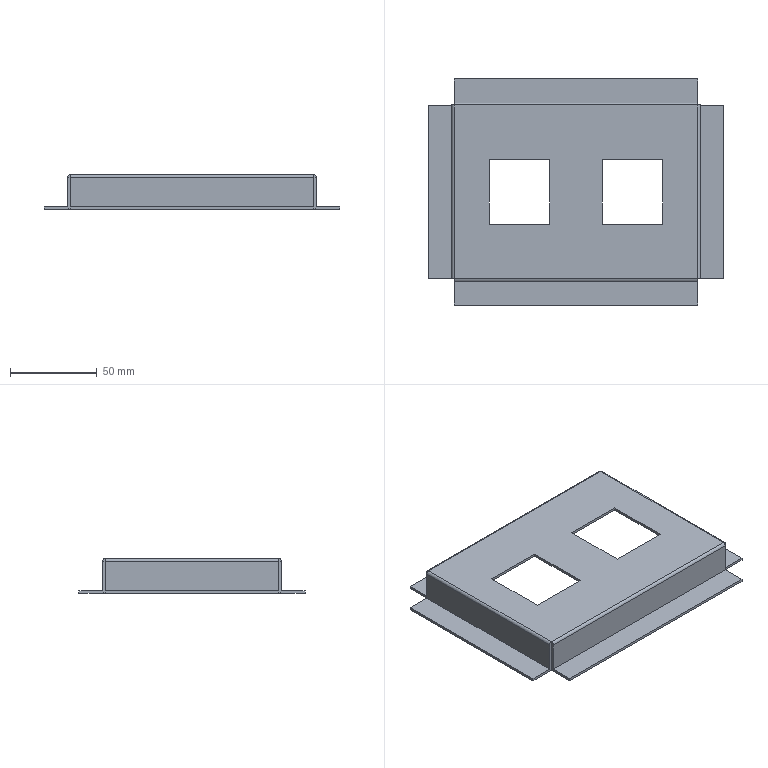Part | NX | features BREP 1 | 1 solid | 58 faces | box 170 x 130 x 20 mm | volume 41003 mm3 | plane 54 | cylinder 4 | commonest cylinder face diameters 3 x4
STEP:
#1=CARTESIAN_POINT('',(-70.,50.,0.));
#2=VERTEX_POINT('',#1);
#3=CARTESIAN_POINT('',(70.,50.,0.));
#4=VERTEX_POINT('',#3);
#5=CARTESIAN_POINT('',(-70.,50.,0.));
#6=DIRECTION('',(1.,0.,0.));
#7=VECTOR('',#6,1000.);
#8=LINE('',#5,#7);
#9=EDGE_CURVE('',#2,#4,#8,.T.);
#10=ORIENTED_EDGE('',*,*,#9,.T.);
#11=CARTESIAN_POINT('',(70.,-50.,0.));
#12=VERTEX_POINT('',#11);
#13=CARTESIAN_POINT('',(70.,50.,0.));
#14=DIRECTION('',(0.,-1.,0.));
#15=VECTOR('',#14,1000.);
#16=LINE('',#13,#15);
#17=EDGE_CURVE('',#4,#12,#16,.T.);
#18=ORIENTED_EDGE('',*,*,#17,.T.);
#19=CARTESIAN_POINT('',(-70.,-50.,0.));
#20=VERTEX_POINT('',#19);
#21=CARTESIAN_POINT('',(70.,-50.,0.));
#22=DIRECTION('',(-1.,0.,0.));
#23=VECTOR('',#22,1000.);
#24=LINE('',#21,#23);
#25=EDGE_CURVE('',#12,#20,#24,.T.);
#26=ORIENTED_EDGE('',*,*,#25,.T.);
#27=CARTESIAN_POINT('',(-70.,-50.,0.));
#28=DIRECTION('',(0.,1.,0.));
#29=VECTOR('',#28,1000.);
#30=LINE('',#27,#29);
#31=EDGE_CURVE('',#20,#2,#30,.T.);
#32=ORIENTED_EDGE('',*,*,#31,.T.);
#33=EDGE_LOOP('',(#10,#18,#26,#32));
#34=FACE_BOUND('',#33,.T.);
#35=CARTESIAN_POINT('',(-15.,18.5,0.));
#36=VERTEX_POINT('',#35);
#37=CARTESIAN_POINT('',(-50.,18.5,0.));
#38=VERTEX_POINT('',#37);
#39=CARTESIAN_POINT('',(-15.,18.5,0.));
#40=DIRECTION('',(-1.,0.,0.));
#41=VECTOR('',#40,1000.);
#42=LINE('',#39,#41);
#43=EDGE_CURVE('',#36,#38,#42,.T.);
#44=ORIENTED_EDGE('',*,*,#43,.T.);
#45=CARTESIAN_POINT('',(-50.,-18.5,0.));
#46=VERTEX_POINT('',#45);
#47=CARTESIAN_POINT('',(-50.,18.5,0.));
#48=DIRECTION('',(0.,-1.,0.));
#49=VECTOR('',#48,1000.);
#50=LINE('',#47,#49);
#51=EDGE_CURVE('',#38,#46,#50,.T.);
#52=ORIENTED_EDGE('',*,*,#51,.T.);
#53=CARTESIAN_POINT('',(-15.,-18.5,0.));
#54=VERTEX_POINT('',#53);
#55=CARTESIAN_POINT('',(-50.,-18.5,0.));
#56=DIRECTION('',(1.,0.,0.));
#57=VECTOR('',#56,1000.);
#58=LINE('',#55,#57);
#59=EDGE_CURVE('',#46,#54,#58,.T.);
#60=ORIENTED_EDGE('',*,*,#59,.T.);
#61=CARTESIAN_POINT('',(-15.,-18.5,0.));
#62=DIRECTION('',(0.,1.,0.));
#63=VECTOR('',#62,1000.);
#64=LINE('',#61,#63);
#65=EDGE_CURVE('',#54,#36,#64,.T.);
#66=ORIENTED_EDGE('',*,*,#65,.T.);
#67=EDGE_LOOP('',(#44,#52,#60,#66));
#68=FACE_BOUND('',#67,.T.);
#69=CARTESIAN_POINT('',(50.,-18.5,0.));
#70=VERTEX_POINT('',#69);
#71=CARTESIAN_POINT('',(15.,-18.5,0.));
#72=VERTEX_POINT('',#71);
#73=CARTESIAN_POINT('',(50.,-18.5,0.));
#74=DIRECTION('',(-1.,0.,0.));
#75=VECTOR('',#74,1000.);
#76=LINE('',#73,#75);
#77=EDGE_CURVE('',#70,#72,#76,.T.);
#78=ORIENTED_EDGE('',*,*,#77,.F.);
#79=CARTESIAN_POINT('',(50.,18.5,0.));
#80=VERTEX_POINT('',#79);
#81=CARTESIAN_POINT('',(50.,18.5,0.));
#82=DIRECTION('',(0.,-1.,0.));
#83=VECTOR('',#82,1000.);
#84=LINE('',#81,#83);
#85=EDGE_CURVE('',#80,#70,#84,.T.);
#86=ORIENTED_EDGE('',*,*,#85,.F.);
#87=CARTESIAN_POINT('',(15.,18.5,0.));
#88=VERTEX_POINT('',#87);
#89=CARTESIAN_POINT('',(15.,18.5,0.));
#90=DIRECTION('',(1.,0.,0.));
#91=VECTOR('',#90,1000.);
#92=LINE('',#89,#91);
#93=EDGE_CURVE('',#88,#80,#92,.T.);
#94=ORIENTED_EDGE('',*,*,#93,.F.);
#95=CARTESIAN_POINT('',(15.,-18.5,0.));
#96=DIRECTION('',(0.,1.,0.));
#97=VECTOR('',#96,1000.);
#98=LINE('',#95,#97);
#99=EDGE_CURVE('',#72,#88,#98,.T.);
#100=ORIENTED_EDGE('',*,*,#99,.F.);
#101=EDGE_LOOP('',(#78,#86,#94,#100));
#102=FACE_BOUND('',#101,.T.);
#103=CARTESIAN_POINT('',(0.,0.,0.));
#104=DIRECTION('',(0.,0.,1.));
#105=DIRECTION('',(1.,0.,0.));
#106=AXIS2_PLACEMENT_3D('',#103,#104,#105);
#107=PLANE('',#106);
#108=ADVANCED_FACE('',(#34,#68,#102),#107,.F.);
#109=CARTESIAN_POINT('',(-70.,-50.,-18.5));
#110=VERTEX_POINT('',#109);
#111=CARTESIAN_POINT('',(-70.,-50.,0.));
#112=DIRECTION('',(0.,0.,-1.));
#113=VECTOR('',#112,1000.);
#114=LINE('',#111,#113);
#115=EDGE_CURVE('',#20,#110,#114,.T.);
#116=ORIENTED_EDGE('',*,*,#115,.T.);
#117=CARTESIAN_POINT('',(-70.,50.,-18.5));
#118=VERTEX_POINT('',#117);
#119=CARTESIAN_POINT('',(-70.,50.,-18.5));
#120=DIRECTION('',(0.,-1.,0.));
#121=VECTOR('',#120,1000.);
#122=LINE('',#119,#121);
#123=EDGE_CURVE('',#118,#110,#122,.T.);
#124=ORIENTED_EDGE('',*,*,#123,.F.);
#125=CARTESIAN_POINT('',(-70.,50.,0.));
#126=DIRECTION('',(0.,0.,-1.));
#127=VECTOR('',#126,1000.);
#128=LINE('',#125,#127);
#129=EDGE_CURVE('',#2,#118,#128,.T.);
#130=ORIENTED_EDGE('',*,*,#129,.F.);
#131=ORIENTED_EDGE('',*,*,#31,.F.);
#132=EDGE_LOOP('',(#116,#124,#130,#131));
#133=FACE_BOUND('',#132,.T.);
#134=CARTESIAN_POINT('',(-70.,-50.,0.));
#135=DIRECTION('',(1.,0.,0.));
#136=DIRECTION('',(0.,1.,0.));
#137=AXIS2_PLACEMENT_3D('',#134,#135,#136);
#138=PLANE('',#137);
#139=ADVANCED_FACE('',(#133),#138,.T.);
#140=CARTESIAN_POINT('',(-71.5,50.,0.));
#141=VERTEX_POINT('',#140);
#142=CARTESIAN_POINT('',(-71.5,50.,0.));
#143=DIRECTION('',(1.,0.,0.));
#144=VECTOR('',#143,1000.);
#145=LINE('',#142,#144);
#146=EDGE_CURVE('',#141,#2,#145,.T.);
#147=ORIENTED_EDGE('',*,*,#146,.T.);
#148=ORIENTED_EDGE('',*,*,#129,.T.);
#149=CARTESIAN_POINT('',(-71.5,50.,-17.));
#150=VERTEX_POINT('',#149);
#151=CARTESIAN_POINT('',(-71.5,50.,-17.));
#152=DIRECTION('',(0.7071,0.,-0.7071));
#153=VECTOR('',#152,1000.);
#154=LINE('',#151,#153);
#155=EDGE_CURVE('',#150,#118,#154,.T.);
#156=ORIENTED_EDGE('',*,*,#155,.F.);
#157=CARTESIAN_POINT('',(-71.5,50.,0.));
#158=DIRECTION('',(0.,0.,-1.));
#159=VECTOR('',#158,1000.);
#160=LINE('',#157,#159);
#161=EDGE_CURVE('',#141,#150,#160,.T.);
#162=ORIENTED_EDGE('',*,*,#161,.F.);
#163=EDGE_LOOP('',(#147,#148,#156,#162));
#164=FACE_BOUND('',#163,.T.);
#165=CARTESIAN_POINT('',(-70.75,50.,-9.25));
#166=DIRECTION('',(0.,1.,0.));
#167=DIRECTION('',(1.,0.,0.));
#168=AXIS2_PLACEMENT_3D('',#165,#166,#167);
#169=PLANE('',#168);
#170=ADVANCED_FACE('',(#164),#169,.T.);
#171=CARTESIAN_POINT('',(-71.5,-50.,0.));
#172=VERTEX_POINT('',#171);
#173=CARTESIAN_POINT('',(-71.5,-50.,0.));
#174=DIRECTION('',(0.,1.,0.));
#175=VECTOR('',#174,1000.);
#176=LINE('',#173,#175);
#177=EDGE_CURVE('',#172,#141,#176,.T.);
#178=ORIENTED_EDGE('',*,*,#177,.T.);
#179=ORIENTED_EDGE('',*,*,#161,.T.);
#180=CARTESIAN_POINT('',(-71.5,-50.,-17.));
#181=VERTEX_POINT('',#180);
#182=CARTESIAN_POINT('',(-71.5,50.,-17.));
#183=DIRECTION('',(0.,-1.,0.));
#184=VECTOR('',#183,1000.);
#185=LINE('',#182,#184);
#186=EDGE_CURVE('',#150,#181,#185,.T.);
#187=ORIENTED_EDGE('',*,*,#186,.T.);
#188=CARTESIAN_POINT('',(-71.5,-50.,0.));
#189=DIRECTION('',(0.,0.,-1.));
#190=VECTOR('',#189,1000.);
#191=LINE('',#188,#190);
#192=EDGE_CURVE('',#172,#181,#191,.T.);
#193=ORIENTED_EDGE('',*,*,#192,.F.);
#194=EDGE_LOOP('',(#178,#179,#187,#193));
#195=FACE_BOUND('',#194,.T.);
#196=CARTESIAN_POINT('',(-71.5,-50.,0.));
#197=DIRECTION('',(1.,0.,0.));
#198=DIRECTION('',(0.,1.,0.));
#199=AXIS2_PLACEMENT_3D('',#196,#197,#198);
#200=PLANE('',#199);
#201=ADVANCED_FACE('',(#195),#200,.F.);
#202=CARTESIAN_POINT('',(-71.5,-50.,-17.));
#203=DIRECTION('',(0.7071,0.,-0.7071));
#204=VECTOR('',#203,1000.);
#205=LINE('',#202,#204);
#206=EDGE_CURVE('',#181,#110,#205,.T.);
#207=ORIENTED_EDGE('',*,*,#206,.T.);
#208=ORIENTED_EDGE('',*,*,#115,.F.);
#209=CARTESIAN_POINT('',(-71.5,-50.,0.));
#210=DIRECTION('',(1.,0.,0.));
#211=VECTOR('',#210,1000.);
#212=LINE('',#209,#211);
#213=EDGE_CURVE('',#172,#20,#212,.T.);
#214=ORIENTED_EDGE('',*,*,#213,.F.);
#215=ORIENTED_EDGE('',*,*,#192,.T.);
#216=EDGE_LOOP('',(#207,#208,#214,#215));
#217=FACE_BOUND('',#216,.T.);
#218=CARTESIAN_POINT('',(-70.75,-50.,-9.25));
#219=DIRECTION('',(0.,1.,0.));
#220=DIRECTION('',(1.,0.,0.));
#221=AXIS2_PLACEMENT_3D('',#218,#219,#220);
#222=PLANE('',#221);
#223=ADVANCED_FACE('',(#217),#222,.F.);
#224=CARTESIAN_POINT('',(-70.,-50.,1.5));
#225=VERTEX_POINT('',#224);
#226=CARTESIAN_POINT('',(-70.,-50.,0.));
#227=DIRECTION('',(0.,0.,1.));
#228=VECTOR('',#227,1000.);
#229=LINE('',#226,#228);
#230=EDGE_CURVE('',#20,#225,#229,.T.);
#231=ORIENTED_EDGE('',*,*,#230,.T.);
#232=CARTESIAN_POINT('',(-70.,-50.,0.));
#233=DIRECTION('',(0.,-1.,0.));
#234=DIRECTION('',(0.,0.,1.));
#235=AXIS2_PLACEMENT_3D('',#232,#233,#234);
#236=CIRCLE('',#235,1.5);
#237=EDGE_CURVE('',#225,#172,#236,.T.);
#238=ORIENTED_EDGE('',*,*,#237,.T.);
#239=ORIENTED_EDGE('',*,*,#213,.T.);
#240=EDGE_LOOP('',(#231,#238,#239));
#241=FACE_BOUND('',#240,.T.);
#242=CARTESIAN_POINT('',(-70.53,-50.,0.5303));
#243=DIRECTION('',(0.,1.,0.));
#244=DIRECTION('',(1.,0.,0.));
#245=AXIS2_PLACEMENT_3D('',#242,#243,#244);
#246=PLANE('',#245);
#247=ADVANCED_FACE('',(#241),#246,.F.);
#248=CARTESIAN_POINT('',(-70.,50.,1.5));
#249=VERTEX_POINT('',#248);
#250=CARTESIAN_POINT('',(-70.,-50.,1.5));
#251=DIRECTION('',(0.,1.,0.));
#252=VECTOR('',#251,1000.);
#253=LINE('',#250,#252);
#254=EDGE_CURVE('',#225,#249,#253,.T.);
#255=ORIENTED_EDGE('',*,*,#254,.T.);
#256=CARTESIAN_POINT('',(-70.,50.,0.));
#257=DIRECTION('',(0.,-1.,0.));
#258=DIRECTION('',(0.,0.,1.));
#259=AXIS2_PLACEMENT_3D('',#256,#257,#258);
#260=CIRCLE('',#259,1.5);
#261=EDGE_CURVE('',#249,#141,#260,.T.);
#262=ORIENTED_EDGE('',*,*,#261,.T.);
#263=ORIENTED_EDGE('',*,*,#177,.F.);
#264=ORIENTED_EDGE('',*,*,#237,.F.);
#265=EDGE_LOOP('',(#255,#262,#263,#264));
#266=FACE_BOUND('',#265,.T.);
#267=CARTESIAN_POINT('',(-70.,-50.,0.));
#268=DIRECTION('',(0.,1.,0.));
#269=DIRECTION('',(-1.,0.,0.));
#270=AXIS2_PLACEMENT_3D('',#267,#268,#269);
#271=CYLINDRICAL_SURFACE('',#270,1.5);
#272=ADVANCED_FACE('',(#266),#271,.T.);
#273=ORIENTED_EDGE('',*,*,#146,.F.);
#274=ORIENTED_EDGE('',*,*,#261,.F.);
#275=CARTESIAN_POINT('',(-70.,50.,0.));
#276=DIRECTION('',(0.,0.,1.));
#277=VECTOR('',#276,1000.);
#278=LINE('',#275,#277);
#279=EDGE_CURVE('',#2,#249,#278,.T.);
#280=ORIENTED_EDGE('',*,*,#279,.F.);
#281=EDGE_LOOP('',(#273,#274,#280));
#282=FACE_BOUND('',#281,.T.);
#283=CARTESIAN_POINT('',(-70.53,50.,0.5303));
#284=DIRECTION('',(0.,1.,0.));
#285=DIRECTION('',(1.,0.,0.));
#286=AXIS2_PLACEMENT_3D('',#283,#284,#285);
#287=PLANE('',#286);
#288=ADVANCED_FACE('',(#282),#287,.T.);
#289=ORIENTED_EDGE('',*,*,#279,.T.);
#290=CARTESIAN_POINT('',(-70.,51.5,0.));
#291=VERTEX_POINT('',#290);
#292=CARTESIAN_POINT('',(-70.,50.,0.));
#293=DIRECTION('',(-1.,0.,0.));
#294=DIRECTION('',(0.,0.,1.));
#295=AXIS2_PLACEMENT_3D('',#292,#293,#294);
#296=CIRCLE('',#295,1.5);
#297=EDGE_CURVE('',#249,#291,#296,.T.);
#298=ORIENTED_EDGE('',*,*,#297,.T.);
#299=CARTESIAN_POINT('',(-70.,51.5,0.));
#300=DIRECTION('',(0.,-1.,0.));
#301=VECTOR('',#300,1000.);
#302=LINE('',#299,#301);
#303=EDGE_CURVE('',#291,#2,#302,.T.);
#304=ORIENTED_EDGE('',*,*,#303,.T.);
#305=EDGE_LOOP('',(#289,#298,#304));
#306=FACE_BOUND('',#305,.T.);
#307=CARTESIAN_POINT('',(-70.,50.53,0.5303));
#308=DIRECTION('',(1.,0.,0.));
#309=DIRECTION('',(0.,1.,0.));
#310=AXIS2_PLACEMENT_3D('',#307,#308,#309);
#311=PLANE('',#310);
#312=ADVANCED_FACE('',(#306),#311,.F.);
#313=CARTESIAN_POINT('',(-70.,51.5,-17.));
#314=VERTEX_POINT('',#313);
#315=CARTESIAN_POINT('',(-70.,50.,-18.5));
#316=VERTEX_POINT('',#315);
#317=CARTESIAN_POINT('',(-70.,51.5,-17.));
#318=DIRECTION('',(0.,-0.7071,-0.7071));
#319=VECTOR('',#318,1000.);
#320=LINE('',#317,#319);
#321=EDGE_CURVE('',#314,#316,#320,.T.);
#322=ORIENTED_EDGE('',*,*,#321,.T.);
#323=CARTESIAN_POINT('',(-70.,50.,0.));
#324=DIRECTION('',(0.,0.,-1.));
#325=VECTOR('',#324,1000.);
#326=LINE('',#323,#325);
#327=EDGE_CURVE('',#2,#316,#326,.T.);
#328=ORIENTED_EDGE('',*,*,#327,.F.);
#329=ORIENTED_EDGE('',*,*,#303,.F.);
#330=CARTESIAN_POINT('',(-70.,51.5,0.));
#331=DIRECTION('',(0.,0.,-1.));
#332=VECTOR('',#331,1000.);
#333=LINE('',#330,#332);
#334=EDGE_CURVE('',#291,#314,#333,.T.);
#335=ORIENTED_EDGE('',*,*,#334,.T.);
#336=EDGE_LOOP('',(#322,#328,#329,#335));
#337=FACE_BOUND('',#336,.T.);
#338=CARTESIAN_POINT('',(-70.,50.75,-9.25));
#339=DIRECTION('',(1.,0.,0.));
#340=DIRECTION('',(0.,1.,0.));
#341=AXIS2_PLACEMENT_3D('',#338,#339,#340);
#342=PLANE('',#341);
#343=ADVANCED_FACE('',(#337),#342,.F.);
#344=CARTESIAN_POINT('',(70.,51.5,0.));
#345=VERTEX_POINT('',#344);
#346=CARTESIAN_POINT('',(-70.,51.5,0.));
#347=DIRECTION('',(1.,0.,0.));
#348=VECTOR('',#347,1000.);
#349=LINE('',#346,#348);
#350=EDGE_CURVE('',#291,#345,#349,.T.);
#351=ORIENTED_EDGE('',*,*,#350,.T.);
#352=CARTESIAN_POINT('',(70.,51.5,-17.));
#353=VERTEX_POINT('',#352);
#354=CARTESIAN_POINT('',(70.,51.5,0.));
#355=DIRECTION('',(0.,0.,-1.));
#356=VECTOR('',#355,1000.);
#357=LINE('',#354,#356);
#358=EDGE_CURVE('',#345,#353,#357,.T.);
#359=ORIENTED_EDGE('',*,*,#358,.T.);
#360=CARTESIAN_POINT('',(70.,51.5,-17.));
#361=DIRECTION('',(-1.,0.,0.));
#362=VECTOR('',#361,1000.);
#363=LINE('',#360,#362);
#364=EDGE_CURVE('',#353,#314,#363,.T.);
#365=ORIENTED_EDGE('',*,*,#364,.T.);
#366=ORIENTED_EDGE('',*,*,#334,.F.);
#367=EDGE_LOOP('',(#351,#359,#365,#366));
#368=FACE_BOUND('',#367,.T.);
#369=CARTESIAN_POINT('',(-70.,51.5,0.));
#370=DIRECTION('',(0.,-1.,0.));
#371=DIRECTION('',(0.,0.,-1.));
#372=AXIS2_PLACEMENT_3D('',#369,#370,#371);
#373=PLANE('',#372);
#374=ADVANCED_FACE('',(#368),#373,.F.);
#375=ORIENTED_EDGE('',*,*,#364,.F.);
#376=CARTESIAN_POINT('',(70.,65.,-17.));
#377=VERTEX_POINT('',#376);
#378=CARTESIAN_POINT('',(70.,65.,-17.));
#379=DIRECTION('',(0.,-1.,0.));
#380=VECTOR('',#379,1000.);
#381=LINE('',#378,#380);
#382=EDGE_CURVE('',#377,#353,#381,.T.);
#383=ORIENTED_EDGE('',*,*,#382,.F.);
#384=CARTESIAN_POINT('',(-70.,65.,-17.));
#385=VERTEX_POINT('',#384);
#386=CARTESIAN_POINT('',(-70.,65.,-17.));
#387=DIRECTION('',(1.,0.,0.));
#388=VECTOR('',#387,1000.);
#389=LINE('',#386,#388);
#390=EDGE_CURVE('',#385,#377,#389,.T.);
#391=ORIENTED_EDGE('',*,*,#390,.F.);
#392=CARTESIAN_POINT('',(-70.,51.5,-17.));
#393=DIRECTION('',(0.,1.,0.));
#394=VECTOR('',#393,1000.);
#395=LINE('',#392,#394);
#396=EDGE_CURVE('',#314,#385,#395,.T.);
#397=ORIENTED_EDGE('',*,*,#396,.F.);
#398=EDGE_LOOP('',(#375,#383,#391,#397));
#399=FACE_BOUND('',#398,.T.);
#400=CARTESIAN_POINT('',(-70.,50.,-17.));
#401=DIRECTION('',(0.,0.,-1.));
#402=DIRECTION('',(0.,-1.,0.));
#403=AXIS2_PLACEMENT_3D('',#400,#401,#402);
#404=PLANE('',#403);
#405=ADVANCED_FACE('',(#399),#404,.F.);
#406=CARTESIAN_POINT('',(-70.,65.,-18.5));
#407=VERTEX_POINT('',#406);
#408=CARTESIAN_POINT('',(-70.,65.,-18.5));
#409=DIRECTION('',(0.,0.,1.));
#410=VECTOR('',#409,1000.);
#411=LINE('',#408,#410);
#412=EDGE_CURVE('',#407,#385,#411,.T.);
#413=ORIENTED_EDGE('',*,*,#412,.F.);
#414=CARTESIAN_POINT('',(-70.,50.,-18.5));
#415=DIRECTION('',(0.,1.,0.));
#416=VECTOR('',#415,1000.);
#417=LINE('',#414,#416);
#418=EDGE_CURVE('',#316,#407,#417,.T.);
#419=ORIENTED_EDGE('',*,*,#418,.F.);
#420=ORIENTED_EDGE('',*,*,#321,.F.);
#421=ORIENTED_EDGE('',*,*,#396,.T.);
#422=EDGE_LOOP('',(#413,#419,#420,#421));
#423=FACE_BOUND('',#422,.T.);
#424=CARTESIAN_POINT('',(-70.,57.5,-17.75));
#425=DIRECTION('',(-1.,0.,0.));
#426=DIRECTION('',(0.,0.,1.));
#427=AXIS2_PLACEMENT_3D('',#424,#425,#426);
#428=PLANE('',#427);
#429=ADVANCED_FACE('',(#423),#428,.T.);
#430=CARTESIAN_POINT('',(70.,65.,-18.5));
#431=VERTEX_POINT('',#430);
#432=CARTESIAN_POINT('',(-70.,65.,-18.5));
#433=DIRECTION('',(1.,0.,0.));
#434=VECTOR('',#433,1000.);
#435=LINE('',#432,#434);
#436=EDGE_CURVE('',#407,#431,#435,.T.);
#437=ORIENTED_EDGE('',*,*,#436,.T.);
#438=CARTESIAN_POINT('',(70.,50.,-18.5));
#439=VERTEX_POINT('',#438);
#440=CARTESIAN_POINT('',(70.,65.,-18.5));
#441=DIRECTION('',(0.,-1.,0.));
#442=VECTOR('',#441,1000.);
#443=LINE('',#440,#442);
#444=EDGE_CURVE('',#431,#439,#443,.T.);
#445=ORIENTED_EDGE('',*,*,#444,.T.);
#446=CARTESIAN_POINT('',(70.,50.,-18.5));
#447=DIRECTION('',(-1.,0.,0.));
#448=VECTOR('',#447,1000.);
#449=LINE('',#446,#448);
#450=EDGE_CURVE('',#439,#316,#449,.T.);
#451=ORIENTED_EDGE('',*,*,#450,.T.);
#452=ORIENTED_EDGE('',*,*,#418,.T.);
#453=EDGE_LOOP('',(#437,#445,#451,#452));
#454=FACE_BOUND('',#453,.T.);
#455=CARTESIAN_POINT('',(-70.,50.,-18.5));
#456=DIRECTION('',(0.,0.,-1.));
#457=DIRECTION('',(0.,-1.,0.));
#458=AXIS2_PLACEMENT_3D('',#455,#456,#457);
#459=PLANE('',#458);
#460=ADVANCED_FACE('',(#454),#459,.T.);
#461=ORIENTED_EDGE('',*,*,#327,.T.);
#462=ORIENTED_EDGE('',*,*,#450,.F.);
#463=CARTESIAN_POINT('',(70.,50.,0.));
#464=DIRECTION('',(0.,0.,-1.));
#465=VECTOR('',#464,1000.);
#466=LINE('',#463,#465);
#467=EDGE_CURVE('',#4,#439,#466,.T.);
#468=ORIENTED_EDGE('',*,*,#467,.F.);
#469=ORIENTED_EDGE('',*,*,#9,.F.);
#470=EDGE_LOOP('',(#461,#462,#468,#469));
#471=FACE_BOUND('',#470,.T.);
#472=CARTESIAN_POINT('',(-70.,50.,0.));
#473=DIRECTION('',(0.,-1.,0.));
#474=DIRECTION('',(0.,0.,-1.));
#475=AXIS2_PLACEMENT_3D('',#472,#473,#474);
#476=PLANE('',#475);
#477=ADVANCED_FACE('',(#471),#476,.T.);
#478=CARTESIAN_POINT('',(70.,51.5,0.));
#479=DIRECTION('',(0.,-1.,0.));
#480=VECTOR('',#479,1000.);
#481=LINE('',#478,#480);
#482=EDGE_CURVE('',#345,#4,#481,.T.);
#483=ORIENTED_EDGE('',*,*,#482,.T.);
#484=ORIENTED_EDGE('',*,*,#467,.T.);
#485=CARTESIAN_POINT('',(70.,51.5,-17.));
#486=DIRECTION('',(0.,-0.7071,-0.7071));
#487=VECTOR('',#486,1000.);
#488=LINE('',#485,#487);
#489=EDGE_CURVE('',#353,#439,#488,.T.);
#490=ORIENTED_EDGE('',*,*,#489,.F.);
#491=ORIENTED_EDGE('',*,*,#358,.F.);
#492=EDGE_LOOP('',(#483,#484,#490,#491));
#493=FACE_BOUND('',#492,.T.);
#494=CARTESIAN_POINT('',(70.,50.75,-9.25));
#495=DIRECTION('',(1.,0.,0.));
#496=DIRECTION('',(0.,1.,0.));
#497=AXIS2_PLACEMENT_3D('',#494,#495,#496);
#498=PLANE('',#497);
#499=ADVANCED_FACE('',(#493),#498,.T.);
#500=ORIENTED_EDGE('',*,*,#489,.T.);
#501=ORIENTED_EDGE('',*,*,#444,.F.);
#502=CARTESIAN_POINT('',(70.,65.,-18.5));
#503=DIRECTION('',(0.,0.,1.));
#504=VECTOR('',#503,1000.);
#505=LINE('',#502,#504);
#506=EDGE_CURVE('',#431,#377,#505,.T.);
#507=ORIENTED_EDGE('',*,*,#506,.T.);
#508=ORIENTED_EDGE('',*,*,#382,.T.);
#509=EDGE_LOOP('',(#500,#501,#507,#508));
#510=FACE_BOUND('',#509,.T.);
#511=CARTESIAN_POINT('',(70.,57.5,-17.75));
#512=DIRECTION('',(1.,0.,0.));
#513=DIRECTION('',(0.,1.,0.));
#514=AXIS2_PLACEMENT_3D('',#511,#512,#513);
#515=PLANE('',#514);
#516=ADVANCED_FACE('',(#510),#515,.T.);
#517=ORIENTED_EDGE('',*,*,#412,.T.);
#518=ORIENTED_EDGE('',*,*,#390,.T.);
#519=ORIENTED_EDGE('',*,*,#506,.F.);
#520=ORIENTED_EDGE('',*,*,#436,.F.);
#521=EDGE_LOOP('',(#517,#518,#519,#520));
#522=FACE_BOUND('',#521,.T.);
#523=CARTESIAN_POINT('',(0.,65.,-17.75));
#524=DIRECTION('',(0.,1.,0.));
#525=DIRECTION('',(1.,0.,0.));
#526=AXIS2_PLACEMENT_3D('',#523,#524,#525);
#527=PLANE('',#526);
#528=ADVANCED_FACE('',(#522),#527,.T.);
#529=ORIENTED_EDGE('',*,*,#482,.F.);
#530=CARTESIAN_POINT('',(70.,50.,1.5));
#531=VERTEX_POINT('',#530);
#532=CARTESIAN_POINT('',(70.,50.,0.));
#533=DIRECTION('',(-1.,0.,0.));
#534=DIRECTION('',(0.,0.,1.));
#535=AXIS2_PLACEMENT_3D('',#532,#533,#534);
#536=CIRCLE('',#535,1.5);
#537=EDGE_CURVE('',#531,#345,#536,.T.);
#538=ORIENTED_EDGE('',*,*,#537,.F.);
#539=CARTESIAN_POINT('',(70.,50.,0.));
#540=DIRECTION('',(0.,0.,1.));
#541=VECTOR('',#540,1000.);
#542=LINE('',#539,#541);
#543=EDGE_CURVE('',#4,#531,#542,.T.);
#544=ORIENTED_EDGE('',*,*,#543,.F.);
#545=EDGE_LOOP('',(#529,#538,#544));
#546=FACE_BOUND('',#545,.T.);
#547=CARTESIAN_POINT('',(70.,50.53,0.5303));
#548=DIRECTION('',(1.,0.,0.));
#549=DIRECTION('',(0.,1.,0.));
#550=AXIS2_PLACEMENT_3D('',#547,#548,#549);
#551=PLANE('',#550);
#552=ADVANCED_FACE('',(#546),#551,.T.);
#553=ORIENTED_EDGE('',*,*,#543,.T.);
#554=CARTESIAN_POINT('',(71.5,50.,0.));
#555=VERTEX_POINT('',#554);
#556=CARTESIAN_POINT('',(70.,50.,0.));
#557=DIRECTION('',(0.,1.,0.));
#558=DIRECTION('',(0.,0.,1.));
#559=AXIS2_PLACEMENT_3D('',#556,#557,#558);
#560=CIRCLE('',#559,1.5);
#561=EDGE_CURVE('',#531,#555,#560,.T.);
#562=ORIENTED_EDGE('',*,*,#561,.T.);
#563=CARTESIAN_POINT('',(71.5,50.,0.));
#564=DIRECTION('',(-1.,0.,0.));
#565=VECTOR('',#564,1000.);
#566=LINE('',#563,#565);
#567=EDGE_CURVE('',#555,#4,#566,.T.);
#568=ORIENTED_EDGE('',*,*,#567,.T.);
#569=EDGE_LOOP('',(#553,#562,#568));
#570=FACE_BOUND('',#569,.T.);
#571=CARTESIAN_POINT('',(70.53,50.,0.5303));
#572=DIRECTION('',(0.,-1.,0.));
#573=DIRECTION('',(0.,0.,-1.));
#574=AXIS2_PLACEMENT_3D('',#571,#572,#573);
#575=PLANE('',#574);
#576=ADVANCED_FACE('',(#570),#575,.F.);
#577=CARTESIAN_POINT('',(71.5,50.,-17.));
#578=VERTEX_POINT('',#577);
#579=CARTESIAN_POINT('',(70.,50.,-18.5));
#580=VERTEX_POINT('',#579);
#581=CARTESIAN_POINT('',(71.5,50.,-17.));
#582=DIRECTION('',(-0.7071,0.,-0.7071));
#583=VECTOR('',#582,1000.);
#584=LINE('',#581,#583);
#585=EDGE_CURVE('',#578,#580,#584,.T.);
#586=ORIENTED_EDGE('',*,*,#585,.T.);
#587=CARTESIAN_POINT('',(70.,50.,0.));
#588=DIRECTION('',(0.,0.,-1.));
#589=VECTOR('',#588,1000.);
#590=LINE('',#587,#589);
#591=EDGE_CURVE('',#4,#580,#590,.T.);
#592=ORIENTED_EDGE('',*,*,#591,.F.);
#593=ORIENTED_EDGE('',*,*,#567,.F.);
#594=CARTESIAN_POINT('',(71.5,50.,0.));
#595=DIRECTION('',(0.,0.,-1.));
#596=VECTOR('',#595,1000.);
#597=LINE('',#594,#596);
#598=EDGE_CURVE('',#555,#578,#597,.T.);
#599=ORIENTED_EDGE('',*,*,#598,.T.);
#600=EDGE_LOOP('',(#586,#592,#593,#599));
#601=FACE_BOUND('',#600,.T.);
#602=CARTESIAN_POINT('',(70.75,50.,-9.25));
#603=DIRECTION('',(0.,-1.,0.));
#604=DIRECTION('',(0.,0.,-1.));
#605=AXIS2_PLACEMENT_3D('',#602,#603,#604);
#606=PLANE('',#605);
#607=ADVANCED_FACE('',(#601),#606,.F.);
#608=CARTESIAN_POINT('',(71.5,-50.,0.));
#609=VERTEX_POINT('',#608);
#610=CARTESIAN_POINT('',(71.5,50.,0.));
#611=DIRECTION('',(0.,-1.,0.));
#612=VECTOR('',#611,1000.);
#613=LINE('',#610,#612);
#614=EDGE_CURVE('',#555,#609,#613,.T.);
#615=ORIENTED_EDGE('',*,*,#614,.T.);
#616=CARTESIAN_POINT('',(71.5,-50.,-17.));
#617=VERTEX_POINT('',#616);
#618=CARTESIAN_POINT('',(71.5,-50.,0.));
#619=DIRECTION('',(0.,0.,-1.));
#620=VECTOR('',#619,1000.);
#621=LINE('',#618,#620);
#622=EDGE_CURVE('',#609,#617,#621,.T.);
#623=ORIENTED_EDGE('',*,*,#622,.T.);
#624=CARTESIAN_POINT('',(71.5,50.,-17.));
#625=DIRECTION('',(0.,-1.,0.));
#626=VECTOR('',#625,1000.);
#627=LINE('',#624,#626);
#628=EDGE_CURVE('',#578,#617,#627,.T.);
#629=ORIENTED_EDGE('',*,*,#628,.F.);
#630=ORIENTED_EDGE('',*,*,#598,.F.);
#631=EDGE_LOOP('',(#615,#623,#629,#630));
#632=FACE_BOUND('',#631,.T.);
#633=CARTESIAN_POINT('',(71.5,50.,0.));
#634=DIRECTION('',(-1.,0.,0.));
#635=DIRECTION('',(0.,0.,1.));
#636=AXIS2_PLACEMENT_3D('',#633,#634,#635);
#637=PLANE('',#636);
#638=ADVANCED_FACE('',(#632),#637,.F.);
#639=CARTESIAN_POINT('',(85.,-50.,-17.));
#640=VERTEX_POINT('',#639);
#641=CARTESIAN_POINT('',(85.,50.,-17.));
#642=VERTEX_POINT('',#641);
#643=CARTESIAN_POINT('',(85.,-50.,-17.));
#644=DIRECTION('',(0.,1.,0.));
#645=VECTOR('',#644,1000.);
#646=LINE('',#643,#645);
#647=EDGE_CURVE('',#640,#642,#646,.T.);
#648=ORIENTED_EDGE('',*,*,#647,.T.);
#649=CARTESIAN_POINT('',(85.,50.,-17.));
#650=DIRECTION('',(-1.,0.,0.));
#651=VECTOR('',#650,1000.);
#652=LINE('',#649,#651);
#653=EDGE_CURVE('',#642,#578,#652,.T.);
#654=ORIENTED_EDGE('',*,*,#653,.T.);
#655=ORIENTED_EDGE('',*,*,#628,.T.);
#656=CARTESIAN_POINT('',(71.5,-50.,-17.));
#657=DIRECTION('',(1.,0.,0.));
#658=VECTOR('',#657,1000.);
#659=LINE('',#656,#658);
#660=EDGE_CURVE('',#617,#640,#659,.T.);
#661=ORIENTED_EDGE('',*,*,#660,.T.);
#662=EDGE_LOOP('',(#648,#654,#655,#661));
#663=FACE_BOUND('',#662,.T.);
#664=CARTESIAN_POINT('',(70.,-50.,-17.));
#665=DIRECTION('',(0.,0.,1.));
#666=DIRECTION('',(1.,0.,0.));
#667=AXIS2_PLACEMENT_3D('',#664,#665,#666);
#668=PLANE('',#667);
#669=ADVANCED_FACE('',(#663),#668,.T.);
#670=CARTESIAN_POINT('',(70.,-50.,-18.5));
#671=VERTEX_POINT('',#670);
#672=CARTESIAN_POINT('',(71.5,-50.,-17.));
#673=DIRECTION('',(-0.7071,0.,-0.7071));
#674=VECTOR('',#673,1000.);
#675=LINE('',#672,#674);
#676=EDGE_CURVE('',#617,#671,#675,.T.);
#677=ORIENTED_EDGE('',*,*,#676,.T.);
#678=CARTESIAN_POINT('',(85.,-50.,-18.5));
#679=VERTEX_POINT('',#678);
#680=CARTESIAN_POINT('',(70.,-50.,-18.5));
#681=DIRECTION('',(1.,0.,0.));
#682=VECTOR('',#681,1000.);
#683=LINE('',#680,#682);
#684=EDGE_CURVE('',#671,#679,#683,.T.);
#685=ORIENTED_EDGE('',*,*,#684,.T.);
#686=CARTESIAN_POINT('',(85.,-50.,-18.5));
#687=DIRECTION('',(0.,0.,1.));
#688=VECTOR('',#687,1000.);
#689=LINE('',#686,#688);
#690=EDGE_CURVE('',#679,#640,#689,.T.);
#691=ORIENTED_EDGE('',*,*,#690,.T.);
#692=ORIENTED_EDGE('',*,*,#660,.F.);
#693=EDGE_LOOP('',(#677,#685,#691,#692));
#694=FACE_BOUND('',#693,.T.);
#695=CARTESIAN_POINT('',(77.5,-50.,-17.75));
#696=DIRECTION('',(0.,1.,0.));
#697=DIRECTION('',(1.,0.,0.));
#698=AXIS2_PLACEMENT_3D('',#695,#696,#697);
#699=PLANE('',#698);
#700=ADVANCED_FACE('',(#694),#699,.F.);
#701=CARTESIAN_POINT('',(85.,50.,-18.5));
#702=VERTEX_POINT('',#701);
#703=CARTESIAN_POINT('',(85.,50.,-18.5));
#704=DIRECTION('',(0.,0.,1.));
#705=VECTOR('',#704,1000.);
#706=LINE('',#703,#705);
#707=EDGE_CURVE('',#702,#642,#706,.T.);
#708=ORIENTED_EDGE('',*,*,#707,.T.);
#709=ORIENTED_EDGE('',*,*,#647,.F.);
#710=ORIENTED_EDGE('',*,*,#690,.F.);
#711=CARTESIAN_POINT('',(85.,-50.,-18.5));
#712=DIRECTION('',(0.,1.,0.));
#713=VECTOR('',#712,1000.);
#714=LINE('',#711,#713);
#715=EDGE_CURVE('',#679,#702,#714,.T.);
#716=ORIENTED_EDGE('',*,*,#715,.T.);
#717=EDGE_LOOP('',(#708,#709,#710,#716));
#718=FACE_BOUND('',#717,.T.);
#719=CARTESIAN_POINT('',(85.,0.,-17.75));
#720=DIRECTION('',(-1.,0.,0.));
#721=DIRECTION('',(0.,0.,1.));
#722=AXIS2_PLACEMENT_3D('',#719,#720,#721);
#723=PLANE('',#722);
#724=ADVANCED_FACE('',(#718),#723,.F.);
#725=CARTESIAN_POINT('',(70.,50.,-18.5));
#726=DIRECTION('',(0.,-1.,0.));
#727=VECTOR('',#726,1000.);
#728=LINE('',#725,#727);
#729=EDGE_CURVE('',#580,#671,#728,.T.);
#730=ORIENTED_EDGE('',*,*,#729,.F.);
#731=CARTESIAN_POINT('',(85.,50.,-18.5));
#732=DIRECTION('',(-1.,0.,0.));
#733=VECTOR('',#732,1000.);
#734=LINE('',#731,#733);
#735=EDGE_CURVE('',#702,#580,#734,.T.);
#736=ORIENTED_EDGE('',*,*,#735,.F.);
#737=ORIENTED_EDGE('',*,*,#715,.F.);
#738=ORIENTED_EDGE('',*,*,#684,.F.);
#739=EDGE_LOOP('',(#730,#736,#737,#738));
#740=FACE_BOUND('',#739,.T.);
#741=CARTESIAN_POINT('',(70.,-50.,-18.5));
#742=DIRECTION('',(0.,0.,1.));
#743=DIRECTION('',(1.,0.,0.));
#744=AXIS2_PLACEMENT_3D('',#741,#742,#743);
#745=PLANE('',#744);
#746=ADVANCED_FACE('',(#740),#745,.F.);
#747=ORIENTED_EDGE('',*,*,#707,.F.);
#748=ORIENTED_EDGE('',*,*,#735,.T.);
#749=ORIENTED_EDGE('',*,*,#585,.F.);
#750=ORIENTED_EDGE('',*,*,#653,.F.);
#751=EDGE_LOOP('',(#747,#748,#749,#750));
#752=FACE_BOUND('',#751,.T.);
#753=CARTESIAN_POINT('',(77.5,50.,-17.75));
#754=DIRECTION('',(0.,-1.,0.));
#755=DIRECTION('',(0.,0.,-1.));
#756=AXIS2_PLACEMENT_3D('',#753,#754,#755);
#757=PLANE('',#756);
#758=ADVANCED_FACE('',(#752),#757,.F.);
#759=ORIENTED_EDGE('',*,*,#591,.T.);
#760=ORIENTED_EDGE('',*,*,#729,.T.);
#761=CARTESIAN_POINT('',(70.,-50.,0.));
#762=DIRECTION('',(0.,0.,-1.));
#763=VECTOR('',#762,1000.);
#764=LINE('',#761,#763);
#765=EDGE_CURVE('',#12,#671,#764,.T.);
#766=ORIENTED_EDGE('',*,*,#765,.F.);
#767=ORIENTED_EDGE('',*,*,#17,.F.);
#768=EDGE_LOOP('',(#759,#760,#766,#767));
#769=FACE_BOUND('',#768,.T.);
#770=CARTESIAN_POINT('',(70.,50.,0.));
#771=DIRECTION('',(-1.,0.,0.));
#772=DIRECTION('',(0.,0.,1.));
#773=AXIS2_PLACEMENT_3D('',#770,#771,#772);
#774=PLANE('',#773);
#775=ADVANCED_FACE('',(#769),#774,.T.);
#776=CARTESIAN_POINT('',(71.5,-50.,0.));
#777=DIRECTION('',(-1.,0.,0.));
#778=VECTOR('',#777,1000.);
#779=LINE('',#776,#778);
#780=EDGE_CURVE('',#609,#12,#779,.T.);
#781=ORIENTED_EDGE('',*,*,#780,.T.);
#782=ORIENTED_EDGE('',*,*,#765,.T.);
#783=ORIENTED_EDGE('',*,*,#676,.F.);
#784=ORIENTED_EDGE('',*,*,#622,.F.);
#785=EDGE_LOOP('',(#781,#782,#783,#784));
#786=FACE_BOUND('',#785,.T.);
#787=CARTESIAN_POINT('',(70.75,-50.,-9.25));
#788=DIRECTION('',(0.,-1.,0.));
#789=DIRECTION('',(0.,0.,-1.));
#790=AXIS2_PLACEMENT_3D('',#787,#788,#789);
#791=PLANE('',#790);
#792=ADVANCED_FACE('',(#786),#791,.T.);
#793=ORIENTED_EDGE('',*,*,#780,.F.);
#794=CARTESIAN_POINT('',(70.,-50.,1.5));
#795=VERTEX_POINT('',#794);
#796=CARTESIAN_POINT('',(70.,-50.,0.));
#797=DIRECTION('',(0.,1.,0.));
#798=DIRECTION('',(0.,0.,1.));
#799=AXIS2_PLACEMENT_3D('',#796,#797,#798);
#800=CIRCLE('',#799,1.5);
#801=EDGE_CURVE('',#795,#609,#800,.T.);
#802=ORIENTED_EDGE('',*,*,#801,.F.);
#803=CARTESIAN_POINT('',(70.,-50.,0.));
#804=DIRECTION('',(0.,0.,1.));
#805=VECTOR('',#804,1000.);
#806=LINE('',#803,#805);
#807=EDGE_CURVE('',#12,#795,#806,.T.);
#808=ORIENTED_EDGE('',*,*,#807,.F.);
#809=EDGE_LOOP('',(#793,#802,#808));
#810=FACE_BOUND('',#809,.T.);
#811=CARTESIAN_POINT('',(70.53,-50.,0.5303));
#812=DIRECTION('',(0.,-1.,0.));
#813=DIRECTION('',(0.,0.,-1.));
#814=AXIS2_PLACEMENT_3D('',#811,#812,#813);
#815=PLANE('',#814);
#816=ADVANCED_FACE('',(#810),#815,.T.);
#817=ORIENTED_EDGE('',*,*,#807,.T.);
#818=CARTESIAN_POINT('',(70.,-51.5,0.));
#819=VERTEX_POINT('',#818);
#820=CARTESIAN_POINT('',(70.,-50.,0.));
#821=DIRECTION('',(1.,0.,0.));
#822=DIRECTION('',(0.,0.,1.));
#823=AXIS2_PLACEMENT_3D('',#820,#821,#822);
#824=CIRCLE('',#823,1.5);
#825=EDGE_CURVE('',#795,#819,#824,.T.);
#826=ORIENTED_EDGE('',*,*,#825,.T.);
#827=CARTESIAN_POINT('',(70.,-51.5,0.));
#828=DIRECTION('',(0.,1.,0.));
#829=VECTOR('',#828,1000.);
#830=LINE('',#827,#829);
#831=EDGE_CURVE('',#819,#12,#830,.T.);
#832=ORIENTED_EDGE('',*,*,#831,.T.);
#833=EDGE_LOOP('',(#817,#826,#832));
#834=FACE_BOUND('',#833,.T.);
#835=CARTESIAN_POINT('',(70.,-50.53,0.5303));
#836=DIRECTION('',(-1.,0.,0.));
#837=DIRECTION('',(0.,0.,1.));
#838=AXIS2_PLACEMENT_3D('',#835,#836,#837);
#839=PLANE('',#838);
#840=ADVANCED_FACE('',(#834),#839,.F.);
#841=CARTESIAN_POINT('',(70.,-51.5,-17.));
#842=VERTEX_POINT('',#841);
#843=CARTESIAN_POINT('',(70.,-50.,-18.5));
#844=VERTEX_POINT('',#843);
#845=CARTESIAN_POINT('',(70.,-51.5,-17.));
#846=DIRECTION('',(0.,0.7071,-0.7071));
#847=VECTOR('',#846,1000.);
#848=LINE('',#845,#847);
#849=EDGE_CURVE('',#842,#844,#848,.T.);
#850=ORIENTED_EDGE('',*,*,#849,.T.);
#851=CARTESIAN_POINT('',(70.,-50.,0.));
#852=DIRECTION('',(0.,0.,-1.));
#853=VECTOR('',#852,1000.);
#854=LINE('',#851,#853);
#855=EDGE_CURVE('',#12,#844,#854,.T.);
#856=ORIENTED_EDGE('',*,*,#855,.F.);
#857=ORIENTED_EDGE('',*,*,#831,.F.);
#858=CARTESIAN_POINT('',(70.,-51.5,0.));
#859=DIRECTION('',(0.,0.,-1.));
#860=VECTOR('',#859,1000.);
#861=LINE('',#858,#860);
#862=EDGE_CURVE('',#819,#842,#861,.T.);
#863=ORIENTED_EDGE('',*,*,#862,.T.);
#864=EDGE_LOOP('',(#850,#856,#857,#863));
#865=FACE_BOUND('',#864,.T.);
#866=CARTESIAN_POINT('',(70.,-50.75,-9.25));
#867=DIRECTION('',(-1.,0.,0.));
#868=DIRECTION('',(0.,0.,1.));
#869=AXIS2_PLACEMENT_3D('',#866,#867,#868);
#870=PLANE('',#869);
#871=ADVANCED_FACE('',(#865),#870,.F.);
#872=CARTESIAN_POINT('',(-70.,-51.5,0.));
#873=VERTEX_POINT('',#872);
#874=CARTESIAN_POINT('',(70.,-51.5,0.));
#875=DIRECTION('',(-1.,0.,0.));
#876=VECTOR('',#875,1000.);
#877=LINE('',#874,#876);
#878=EDGE_CURVE('',#819,#873,#877,.T.);
#879=ORIENTED_EDGE('',*,*,#878,.T.);
#880=CARTESIAN_POINT('',(-70.,-51.5,-17.));
#881=VERTEX_POINT('',#880);
#882=CARTESIAN_POINT('',(-70.,-51.5,0.));
#883=DIRECTION('',(0.,0.,-1.));
#884=VECTOR('',#883,1000.);
#885=LINE('',#882,#884);
#886=EDGE_CURVE('',#873,#881,#885,.T.);
#887=ORIENTED_EDGE('',*,*,#886,.T.);
#888=CARTESIAN_POINT('',(70.,-51.5,-17.));
#889=DIRECTION('',(-1.,0.,0.));
#890=VECTOR('',#889,1000.);
#891=LINE('',#888,#890);
#892=EDGE_CURVE('',#842,#881,#891,.T.);
#893=ORIENTED_EDGE('',*,*,#892,.F.);
#894=ORIENTED_EDGE('',*,*,#862,.F.);
#895=EDGE_LOOP('',(#879,#887,#893,#894));
#896=FACE_BOUND('',#895,.T.);
#897=CARTESIAN_POINT('',(70.,-51.5,0.));
#898=DIRECTION('',(0.,1.,0.));
#899=DIRECTION('',(1.,0.,0.));
#900=AXIS2_PLACEMENT_3D('',#897,#898,#899);
#901=PLANE('',#900);
#902=ADVANCED_FACE('',(#896),#901,.F.);
#903=CARTESIAN_POINT('',(-70.,-65.,-17.));
#904=VERTEX_POINT('',#903);
#905=CARTESIAN_POINT('',(70.,-65.,-17.));
#906=VERTEX_POINT('',#905);
#907=CARTESIAN_POINT('',(-70.,-65.,-17.));
#908=DIRECTION('',(1.,0.,0.));
#909=VECTOR('',#908,1000.);
#910=LINE('',#907,#909);
#911=EDGE_CURVE('',#904,#906,#910,.T.);
#912=ORIENTED_EDGE('',*,*,#911,.T.);
#913=CARTESIAN_POINT('',(70.,-65.,-17.));
#914=DIRECTION('',(0.,1.,0.));
#915=VECTOR('',#914,1000.);
#916=LINE('',#913,#915);
#917=EDGE_CURVE('',#906,#842,#916,.T.);
#918=ORIENTED_EDGE('',*,*,#917,.T.);
#919=ORIENTED_EDGE('',*,*,#892,.T.);
#920=CARTESIAN_POINT('',(-70.,-51.5,-17.));
#921=DIRECTION('',(0.,-1.,0.));
#922=VECTOR('',#921,1000.);
#923=LINE('',#920,#922);
#924=EDGE_CURVE('',#881,#904,#923,.T.);
#925=ORIENTED_EDGE('',*,*,#924,.T.);
#926=EDGE_LOOP('',(#912,#918,#919,#925));
#927=FACE_BOUND('',#926,.T.);
#928=CARTESIAN_POINT('',(-70.,-50.,-17.));
#929=DIRECTION('',(0.,0.,1.));
#930=DIRECTION('',(1.,0.,0.));
#931=AXIS2_PLACEMENT_3D('',#928,#929,#930);
#932=PLANE('',#931);
#933=ADVANCED_FACE('',(#927),#932,.T.);
#934=CARTESIAN_POINT('',(-70.,-50.,-18.5));
#935=VERTEX_POINT('',#934);
#936=CARTESIAN_POINT('',(-70.,-51.5,-17.));
#937=DIRECTION('',(0.,0.7071,-0.7071));
#938=VECTOR('',#937,1000.);
#939=LINE('',#936,#938);
#940=EDGE_CURVE('',#881,#935,#939,.T.);
#941=ORIENTED_EDGE('',*,*,#940,.T.);
#942=CARTESIAN_POINT('',(-70.,-65.,-18.5));
#943=VERTEX_POINT('',#942);
#944=CARTESIAN_POINT('',(-70.,-50.,-18.5));
#945=DIRECTION('',(0.,-1.,0.));
#946=VECTOR('',#945,1000.);
#947=LINE('',#944,#946);
#948=EDGE_CURVE('',#935,#943,#947,.T.);
#949=ORIENTED_EDGE('',*,*,#948,.T.);
#950=CARTESIAN_POINT('',(-70.,-65.,-18.5));
#951=DIRECTION('',(0.,0.,1.));
#952=VECTOR('',#951,1000.);
#953=LINE('',#950,#952);
#954=EDGE_CURVE('',#943,#904,#953,.T.);
#955=ORIENTED_EDGE('',*,*,#954,.T.);
#956=ORIENTED_EDGE('',*,*,#924,.F.);
#957=EDGE_LOOP('',(#941,#949,#955,#956));
#958=FACE_BOUND('',#957,.T.);
#959=CARTESIAN_POINT('',(-70.,-57.5,-17.75));
#960=DIRECTION('',(1.,0.,0.));
#961=DIRECTION('',(0.,1.,0.));
#962=AXIS2_PLACEMENT_3D('',#959,#960,#961);
#963=PLANE('',#962);
#964=ADVANCED_FACE('',(#958),#963,.F.);
#965=CARTESIAN_POINT('',(70.,-65.,-18.5));
#966=VERTEX_POINT('',#965);
#967=CARTESIAN_POINT('',(70.,-65.,-18.5));
#968=DIRECTION('',(0.,0.,1.));
#969=VECTOR('',#968,1000.);
#970=LINE('',#967,#969);
#971=EDGE_CURVE('',#966,#906,#970,.T.);
#972=ORIENTED_EDGE('',*,*,#971,.T.);
#973=ORIENTED_EDGE('',*,*,#911,.F.);
#974=ORIENTED_EDGE('',*,*,#954,.F.);
#975=CARTESIAN_POINT('',(-70.,-65.,-18.5));
#976=DIRECTION('',(1.,0.,0.));
#977=VECTOR('',#976,1000.);
#978=LINE('',#975,#977);
#979=EDGE_CURVE('',#943,#966,#978,.T.);
#980=ORIENTED_EDGE('',*,*,#979,.T.);
#981=EDGE_LOOP('',(#972,#973,#974,#980));
#982=FACE_BOUND('',#981,.T.);
#983=CARTESIAN_POINT('',(0.,-65.,-17.75));
#984=DIRECTION('',(0.,1.,0.));
#985=DIRECTION('',(1.,0.,0.));
#986=AXIS2_PLACEMENT_3D('',#983,#984,#985);
#987=PLANE('',#986);
#988=ADVANCED_FACE('',(#982),#987,.F.);
#989=CARTESIAN_POINT('',(70.,-50.,-18.5));
#990=DIRECTION('',(-1.,0.,0.));
#991=VECTOR('',#990,1000.);
#992=LINE('',#989,#991);
#993=EDGE_CURVE('',#844,#935,#992,.T.);
#994=ORIENTED_EDGE('',*,*,#993,.F.);
#995=CARTESIAN_POINT('',(70.,-65.,-18.5));
#996=DIRECTION('',(0.,1.,0.));
#997=VECTOR('',#996,1000.);
#998=LINE('',#995,#997);
#999=EDGE_CURVE('',#966,#844,#998,.T.);
#1000=ORIENTED_EDGE('',*,*,#999,.F.);
#1001=ORIENTED_EDGE('',*,*,#979,.F.);
#1002=ORIENTED_EDGE('',*,*,#948,.F.);
#1003=EDGE_LOOP('',(#994,#1000,#1001,#1002));
#1004=FACE_BOUND('',#1003,.T.);
#1005=CARTESIAN_POINT('',(-70.,-50.,-18.5));
#1006=DIRECTION('',(0.,0.,1.));
#1007=DIRECTION('',(1.,0.,0.));
#1008=AXIS2_PLACEMENT_3D('',#1005,#1006,#1007);
#1009=PLANE('',#1008);
#1010=ADVANCED_FACE('',(#1004),#1009,.F.);
#1011=ORIENTED_EDGE('',*,*,#971,.F.);
#1012=ORIENTED_EDGE('',*,*,#999,.T.);
#1013=ORIENTED_EDGE('',*,*,#849,.F.);
#1014=ORIENTED_EDGE('',*,*,#917,.F.);
#1015=EDGE_LOOP('',(#1011,#1012,#1013,#1014));
#1016=FACE_BOUND('',#1015,.T.);
#1017=CARTESIAN_POINT('',(70.,-57.5,-17.75));
#1018=DIRECTION('',(-1.,0.,0.));
#1019=DIRECTION('',(0.,0.,1.));
#1020=AXIS2_PLACEMENT_3D('',#1017,#1018,#1019);
#1021=PLANE('',#1020);
#1022=ADVANCED_FACE('',(#1016),#1021,.F.);
#1023=ORIENTED_EDGE('',*,*,#855,.T.);
#1024=ORIENTED_EDGE('',*,*,#993,.T.);
#1025=CARTESIAN_POINT('',(-70.,-50.,0.));
#1026=DIRECTION('',(0.,0.,-1.));
#1027=VECTOR('',#1026,1000.);
#1028=LINE('',#1025,#1027);
#1029=EDGE_CURVE('',#20,#935,#1028,.T.);
#1030=ORIENTED_EDGE('',*,*,#1029,.F.);
#1031=ORIENTED_EDGE('',*,*,#25,.F.);
#1032=EDGE_LOOP('',(#1023,#1024,#1030,#1031));
#1033=FACE_BOUND('',#1032,.T.);
#1034=CARTESIAN_POINT('',(70.,-50.,0.));
#1035=DIRECTION('',(0.,1.,0.));
#1036=DIRECTION('',(1.,0.,0.));
#1037=AXIS2_PLACEMENT_3D('',#1034,#1035,#1036);
#1038=PLANE('',#1037);
#1039=ADVANCED_FACE('',(#1033),#1038,.T.);
#1040=CARTESIAN_POINT('',(-70.,-51.5,0.));
#1041=DIRECTION('',(0.,1.,0.));
#1042=VECTOR('',#1041,1000.);
#1043=LINE('',#1040,#1042);
#1044=EDGE_CURVE('',#873,#20,#1043,.T.);
#1045=ORIENTED_EDGE('',*,*,#1044,.T.);
#1046=ORIENTED_EDGE('',*,*,#1029,.T.);
#1047=ORIENTED_EDGE('',*,*,#940,.F.);
#1048=ORIENTED_EDGE('',*,*,#886,.F.);
#1049=EDGE_LOOP('',(#1045,#1046,#1047,#1048));
#1050=FACE_BOUND('',#1049,.T.);
#1051=CARTESIAN_POINT('',(-70.,-50.75,-9.25));
#1052=DIRECTION('',(-1.,0.,0.));
#1053=DIRECTION('',(0.,0.,1.));
#1054=AXIS2_PLACEMENT_3D('',#1051,#1052,#1053);
#1055=PLANE('',#1054);
#1056=ADVANCED_FACE('',(#1050),#1055,.T.);
#1057=ORIENTED_EDGE('',*,*,#1044,.F.);
#1058=CARTESIAN_POINT('',(-70.,-50.,0.));
#1059=DIRECTION('',(1.,0.,0.));
#1060=DIRECTION('',(0.,0.,1.));
#1061=AXIS2_PLACEMENT_3D('',#1058,#1059,#1060);
#1062=CIRCLE('',#1061,1.5);
#1063=EDGE_CURVE('',#225,#873,#1062,.T.);
#1064=ORIENTED_EDGE('',*,*,#1063,.F.);
#1065=ORIENTED_EDGE('',*,*,#230,.F.);
#1066=EDGE_LOOP('',(#1057,#1064,#1065));
#1067=FACE_BOUND('',#1066,.T.);
#1068=CARTESIAN_POINT('',(-70.,-50.53,0.5303));
#1069=DIRECTION('',(-1.,0.,0.));
#1070=DIRECTION('',(0.,0.,1.));
#1071=AXIS2_PLACEMENT_3D('',#1068,#1069,#1070);
#1072=PLANE('',#1071);
#1073=ADVANCED_FACE('',(#1067),#1072,.T.);
#1074=CARTESIAN_POINT('',(70.,-50.,1.5));
#1075=DIRECTION('',(-1.,0.,0.));
#1076=VECTOR('',#1075,1000.);
#1077=LINE('',#1074,#1076);
#1078=EDGE_CURVE('',#795,#225,#1077,.T.);
#1079=ORIENTED_EDGE('',*,*,#1078,.T.);
#1080=ORIENTED_EDGE('',*,*,#1063,.T.);
#1081=ORIENTED_EDGE('',*,*,#878,.F.);
#1082=ORIENTED_EDGE('',*,*,#825,.F.);
#1083=EDGE_LOOP('',(#1079,#1080,#1081,#1082));
#1084=FACE_BOUND('',#1083,.T.);
#1085=CARTESIAN_POINT('',(70.,-50.,0.));
#1086=DIRECTION('',(-1.,0.,0.));
#1087=DIRECTION('',(0.,-1.,0.));
#1088=AXIS2_PLACEMENT_3D('',#1085,#1086,#1087);
#1089=CYLINDRICAL_SURFACE('',#1088,1.5);
#1090=ADVANCED_FACE('',(#1084),#1089,.T.);
#1091=ORIENTED_EDGE('',*,*,#254,.F.);
#1092=ORIENTED_EDGE('',*,*,#1078,.F.);
#1093=CARTESIAN_POINT('',(70.,50.,1.5));
#1094=DIRECTION('',(0.,-1.,0.));
#1095=VECTOR('',#1094,1000.);
#1096=LINE('',#1093,#1095);
#1097=EDGE_CURVE('',#531,#795,#1096,.T.);
#1098=ORIENTED_EDGE('',*,*,#1097,.F.);
#1099=CARTESIAN_POINT('',(-70.,50.,1.5));
#1100=DIRECTION('',(1.,0.,0.));
#1101=VECTOR('',#1100,1000.);
#1102=LINE('',#1099,#1101);
#1103=EDGE_CURVE('',#249,#531,#1102,.T.);
#1104=ORIENTED_EDGE('',*,*,#1103,.F.);
#1105=EDGE_LOOP('',(#1091,#1092,#1098,#1104));
#1106=FACE_BOUND('',#1105,.T.);
#1107=CARTESIAN_POINT('',(-50.,-18.5,1.5));
#1108=VERTEX_POINT('',#1107);
#1109=CARTESIAN_POINT('',(-15.,-18.5,1.5));
#1110=VERTEX_POINT('',#1109);
#1111=CARTESIAN_POINT('',(-50.,-18.5,1.5));
#1112=DIRECTION('',(1.,0.,0.));
#1113=VECTOR('',#1112,1000.);
#1114=LINE('',#1111,#1113);
#1115=EDGE_CURVE('',#1108,#1110,#1114,.T.);
#1116=ORIENTED_EDGE('',*,*,#1115,.F.);
#1117=CARTESIAN_POINT('',(-50.,18.5,1.5));
#1118=VERTEX_POINT('',#1117);
#1119=CARTESIAN_POINT('',(-50.,18.5,1.5));
#1120=DIRECTION('',(0.,-1.,0.));
#1121=VECTOR('',#1120,1000.);
#1122=LINE('',#1119,#1121);
#1123=EDGE_CURVE('',#1118,#1108,#1122,.T.);
#1124=ORIENTED_EDGE('',*,*,#1123,.F.);
#1125=CARTESIAN_POINT('',(-15.,18.5,1.5));
#1126=VERTEX_POINT('',#1125);
#1127=CARTESIAN_POINT('',(-15.,18.5,1.5));
#1128=DIRECTION('',(-1.,0.,0.));
#1129=VECTOR('',#1128,1000.);
#1130=LINE('',#1127,#1129);
#1131=EDGE_CURVE('',#1126,#1118,#1130,.T.);
#1132=ORIENTED_EDGE('',*,*,#1131,.F.);
#1133=CARTESIAN_POINT('',(-15.,-18.5,1.5));
#1134=DIRECTION('',(0.,1.,0.));
#1135=VECTOR('',#1134,1000.);
#1136=LINE('',#1133,#1135);
#1137=EDGE_CURVE('',#1110,#1126,#1136,.T.);
#1138=ORIENTED_EDGE('',*,*,#1137,.F.);
#1139=EDGE_LOOP('',(#1116,#1124,#1132,#1138));
#1140=FACE_BOUND('',#1139,.T.);
#1141=CARTESIAN_POINT('',(15.,18.5,1.5));
#1142=VERTEX_POINT('',#1141);
#1143=CARTESIAN_POINT('',(50.,18.5,1.5));
#1144=VERTEX_POINT('',#1143);
#1145=CARTESIAN_POINT('',(15.,18.5,1.5));
#1146=DIRECTION('',(1.,0.,0.));
#1147=VECTOR('',#1146,1000.);
#1148=LINE('',#1145,#1147);
#1149=EDGE_CURVE('',#1142,#1144,#1148,.T.);
#1150=ORIENTED_EDGE('',*,*,#1149,.T.);
#1151=CARTESIAN_POINT('',(50.,-18.5,1.5));
#1152=VERTEX_POINT('',#1151);
#1153=CARTESIAN_POINT('',(50.,18.5,1.5));
#1154=DIRECTION('',(0.,-1.,0.));
#1155=VECTOR('',#1154,1000.);
#1156=LINE('',#1153,#1155);
#1157=EDGE_CURVE('',#1144,#1152,#1156,.T.);
#1158=ORIENTED_EDGE('',*,*,#1157,.T.);
#1159=CARTESIAN_POINT('',(15.,-18.5,1.5));
#1160=VERTEX_POINT('',#1159);
#1161=CARTESIAN_POINT('',(50.,-18.5,1.5));
#1162=DIRECTION('',(-1.,0.,0.));
#1163=VECTOR('',#1162,1000.);
#1164=LINE('',#1161,#1163);
#1165=EDGE_CURVE('',#1152,#1160,#1164,.T.);
#1166=ORIENTED_EDGE('',*,*,#1165,.T.);
#1167=CARTESIAN_POINT('',(15.,-18.5,1.5));
#1168=DIRECTION('',(0.,1.,0.));
#1169=VECTOR('',#1168,1000.);
#1170=LINE('',#1167,#1169);
#1171=EDGE_CURVE('',#1160,#1142,#1170,.T.);
#1172=ORIENTED_EDGE('',*,*,#1171,.T.);
#1173=EDGE_LOOP('',(#1150,#1158,#1166,#1172));
#1174=FACE_BOUND('',#1173,.T.);
#1175=CARTESIAN_POINT('',(0.,0.,1.5));
#1176=DIRECTION('',(0.,0.,1.));
#1177=DIRECTION('',(1.,0.,0.));
#1178=AXIS2_PLACEMENT_3D('',#1175,#1176,#1177);
#1179=PLANE('',#1178);
#1180=ADVANCED_FACE('',(#1106,#1140,#1174),#1179,.T.);
#1181=ORIENTED_EDGE('',*,*,#1103,.T.);
#1182=ORIENTED_EDGE('',*,*,#537,.T.);
#1183=ORIENTED_EDGE('',*,*,#350,.F.);
#1184=ORIENTED_EDGE('',*,*,#297,.F.);
#1185=EDGE_LOOP('',(#1181,#1182,#1183,#1184));
#1186=FACE_BOUND('',#1185,.T.);
#1187=CARTESIAN_POINT('',(-70.,50.,0.));
#1188=DIRECTION('',(1.,0.,0.));
#1189=DIRECTION('',(0.,1.,0.));
#1190=AXIS2_PLACEMENT_3D('',#1187,#1188,#1189);
#1191=CYLINDRICAL_SURFACE('',#1190,1.5);
#1192=ADVANCED_FACE('',(#1186),#1191,.T.);
#1193=ORIENTED_EDGE('',*,*,#1097,.T.);
#1194=ORIENTED_EDGE('',*,*,#801,.T.);
#1195=ORIENTED_EDGE('',*,*,#614,.F.);
#1196=ORIENTED_EDGE('',*,*,#561,.F.);
#1197=EDGE_LOOP('',(#1193,#1194,#1195,#1196));
#1198=FACE_BOUND('',#1197,.T.);
#1199=CARTESIAN_POINT('',(70.,50.,0.));
#1200=DIRECTION('',(0.,-1.,0.));
#1201=DIRECTION('',(1.,0.,0.));
#1202=AXIS2_PLACEMENT_3D('',#1199,#1200,#1201);
#1203=CYLINDRICAL_SURFACE('',#1202,1.5);
#1204=ADVANCED_FACE('',(#1198),#1203,.T.);
#1205=CARTESIAN_POINT('',(-15.,-18.5,0.));
#1206=DIRECTION('',(0.,0.,1.));
#1207=VECTOR('',#1206,1000.);
#1208=LINE('',#1205,#1207);
#1209=EDGE_CURVE('',#54,#1110,#1208,.T.);
#1210=ORIENTED_EDGE('',*,*,#1209,.T.);
#1211=ORIENTED_EDGE('',*,*,#1137,.T.);
#1212=CARTESIAN_POINT('',(-15.,18.5,0.));
#1213=DIRECTION('',(0.,0.,1.));
#1214=VECTOR('',#1213,1000.);
#1215=LINE('',#1212,#1214);
#1216=EDGE_CURVE('',#36,#1126,#1215,.T.);
#1217=ORIENTED_EDGE('',*,*,#1216,.F.);
#1218=ORIENTED_EDGE('',*,*,#65,.F.);
#1219=EDGE_LOOP('',(#1210,#1211,#1217,#1218));
#1220=FACE_BOUND('',#1219,.T.);
#1221=CARTESIAN_POINT('',(-15.,0.,0.75));
#1222=DIRECTION('',(-1.,0.,0.));
#1223=DIRECTION('',(0.,0.,1.));
#1224=AXIS2_PLACEMENT_3D('',#1221,#1222,#1223);
#1225=PLANE('',#1224);
#1226=ADVANCED_FACE('',(#1220),#1225,.T.);
#1227=ORIENTED_EDGE('',*,*,#1216,.T.);
#1228=ORIENTED_EDGE('',*,*,#1131,.T.);
#1229=CARTESIAN_POINT('',(-50.,18.5,0.));
#1230=DIRECTION('',(0.,0.,1.));
#1231=VECTOR('',#1230,1000.);
#1232=LINE('',#1229,#1231);
#1233=EDGE_CURVE('',#38,#1118,#1232,.T.);
#1234=ORIENTED_EDGE('',*,*,#1233,.F.);
#1235=ORIENTED_EDGE('',*,*,#43,.F.);
#1236=EDGE_LOOP('',(#1227,#1228,#1234,#1235));
#1237=FACE_BOUND('',#1236,.T.);
#1238=CARTESIAN_POINT('',(-32.5,18.5,0.75));
#1239=DIRECTION('',(0.,-1.,0.));
#1240=DIRECTION('',(0.,0.,-1.));
#1241=AXIS2_PLACEMENT_3D('',#1238,#1239,#1240);
#1242=PLANE('',#1241);
#1243=ADVANCED_FACE('',(#1237),#1242,.T.);
#1244=ORIENTED_EDGE('',*,*,#1233,.T.);
#1245=ORIENTED_EDGE('',*,*,#1123,.T.);
#1246=CARTESIAN_POINT('',(-50.,-18.5,0.));
#1247=DIRECTION('',(0.,0.,1.));
#1248=VECTOR('',#1247,1000.);
#1249=LINE('',#1246,#1248);
#1250=EDGE_CURVE('',#46,#1108,#1249,.T.);
#1251=ORIENTED_EDGE('',*,*,#1250,.F.);
#1252=ORIENTED_EDGE('',*,*,#51,.F.);
#1253=EDGE_LOOP('',(#1244,#1245,#1251,#1252));
#1254=FACE_BOUND('',#1253,.T.);
#1255=CARTESIAN_POINT('',(-50.,0.,0.75));
#1256=DIRECTION('',(1.,0.,0.));
#1257=DIRECTION('',(0.,1.,0.));
#1258=AXIS2_PLACEMENT_3D('',#1255,#1256,#1257);
#1259=PLANE('',#1258);
#1260=ADVANCED_FACE('',(#1254),#1259,.T.);
#1261=ORIENTED_EDGE('',*,*,#1250,.T.);
#1262=ORIENTED_EDGE('',*,*,#1115,.T.);
#1263=ORIENTED_EDGE('',*,*,#1209,.F.);
#1264=ORIENTED_EDGE('',*,*,#59,.F.);
#1265=EDGE_LOOP('',(#1261,#1262,#1263,#1264));
#1266=FACE_BOUND('',#1265,.T.);
#1267=CARTESIAN_POINT('',(-32.5,-18.5,0.75));
#1268=DIRECTION('',(0.,1.,0.));
#1269=DIRECTION('',(1.,0.,0.));
#1270=AXIS2_PLACEMENT_3D('',#1267,#1268,#1269);
#1271=PLANE('',#1270);
#1272=ADVANCED_FACE('',(#1266),#1271,.T.);
#1273=CARTESIAN_POINT('',(15.,18.5,0.));
#1274=DIRECTION('',(0.,0.,1.));
#1275=VECTOR('',#1274,1000.);
#1276=LINE('',#1273,#1275);
#1277=EDGE_CURVE('',#88,#1142,#1276,.T.);
#1278=ORIENTED_EDGE('',*,*,#1277,.T.);
#1279=ORIENTED_EDGE('',*,*,#1171,.F.);
#1280=CARTESIAN_POINT('',(15.,-18.5,0.));
#1281=DIRECTION('',(0.,0.,1.));
#1282=VECTOR('',#1281,1000.);
#1283=LINE('',#1280,#1282);
#1284=EDGE_CURVE('',#72,#1160,#1283,.T.);
#1285=ORIENTED_EDGE('',*,*,#1284,.F.);
#1286=ORIENTED_EDGE('',*,*,#99,.T.);
#1287=EDGE_LOOP('',(#1278,#1279,#1285,#1286));
#1288=FACE_BOUND('',#1287,.T.);
#1289=CARTESIAN_POINT('',(15.,0.,0.75));
#1290=DIRECTION('',(-1.,0.,0.));
#1291=DIRECTION('',(0.,0.,1.));
#1292=AXIS2_PLACEMENT_3D('',#1289,#1290,#1291);
#1293=PLANE('',#1292);
#1294=ADVANCED_FACE('',(#1288),#1293,.F.);
#1295=ORIENTED_EDGE('',*,*,#1284,.T.);
#1296=ORIENTED_EDGE('',*,*,#1165,.F.);
#1297=CARTESIAN_POINT('',(50.,-18.5,0.));
#1298=DIRECTION('',(0.,0.,1.));
#1299=VECTOR('',#1298,1000.);
#1300=LINE('',#1297,#1299);
#1301=EDGE_CURVE('',#70,#1152,#1300,.T.);
#1302=ORIENTED_EDGE('',*,*,#1301,.F.);
#1303=ORIENTED_EDGE('',*,*,#77,.T.);
#1304=EDGE_LOOP('',(#1295,#1296,#1302,#1303));
#1305=FACE_BOUND('',#1304,.T.);
#1306=CARTESIAN_POINT('',(32.5,-18.5,0.75));
#1307=DIRECTION('',(0.,-1.,0.));
#1308=DIRECTION('',(0.,0.,-1.));
#1309=AXIS2_PLACEMENT_3D('',#1306,#1307,#1308);
#1310=PLANE('',#1309);
#1311=ADVANCED_FACE('',(#1305),#1310,.F.);
#1312=ORIENTED_EDGE('',*,*,#1301,.T.);
#1313=ORIENTED_EDGE('',*,*,#1157,.F.);
#1314=CARTESIAN_POINT('',(50.,18.5,0.));
#1315=DIRECTION('',(0.,0.,1.));
#1316=VECTOR('',#1315,1000.);
#1317=LINE('',#1314,#1316);
#1318=EDGE_CURVE('',#80,#1144,#1317,.T.);
#1319=ORIENTED_EDGE('',*,*,#1318,.F.);
#1320=ORIENTED_EDGE('',*,*,#85,.T.);
#1321=EDGE_LOOP('',(#1312,#1313,#1319,#1320));
#1322=FACE_BOUND('',#1321,.T.);
#1323=CARTESIAN_POINT('',(50.,0.,0.75));
#1324=DIRECTION('',(1.,0.,0.));
#1325=DIRECTION('',(0.,1.,0.));
#1326=AXIS2_PLACEMENT_3D('',#1323,#1324,#1325);
#1327=PLANE('',#1326);
#1328=ADVANCED_FACE('',(#1322),#1327,.F.);
#1329=ORIENTED_EDGE('',*,*,#1318,.T.);
#1330=ORIENTED_EDGE('',*,*,#1149,.F.);
#1331=ORIENTED_EDGE('',*,*,#1277,.F.);
#1332=ORIENTED_EDGE('',*,*,#93,.T.);
#1333=EDGE_LOOP('',(#1329,#1330,#1331,#1332));
#1334=FACE_BOUND('',#1333,.T.);
#1335=CARTESIAN_POINT('',(32.5,18.5,0.75));
#1336=DIRECTION('',(0.,1.,0.));
#1337=DIRECTION('',(1.,0.,0.));
#1338=AXIS2_PLACEMENT_3D('',#1335,#1336,#1337);
#1339=PLANE('',#1338);
#1340=ADVANCED_FACE('',(#1334),#1339,.F.);
#1341=CARTESIAN_POINT('',(-85.,-50.,-18.5));
#1342=VERTEX_POINT('',#1341);
#1343=CARTESIAN_POINT('',(-85.,-50.,-17.));
#1344=VERTEX_POINT('',#1343);
#1345=CARTESIAN_POINT('',(-85.,-50.,-18.5));
#1346=DIRECTION('',(0.,0.,1.));
#1347=VECTOR('',#1346,1000.);
#1348=LINE('',#1345,#1347);
#1349=EDGE_CURVE('',#1342,#1344,#1348,.T.);
#1350=ORIENTED_EDGE('',*,*,#1349,.F.);
#1351=CARTESIAN_POINT('',(-70.,-50.,-18.5));
#1352=DIRECTION('',(-1.,0.,0.));
#1353=VECTOR('',#1352,1000.);
#1354=LINE('',#1351,#1353);
#1355=EDGE_CURVE('',#110,#1342,#1354,.T.);
#1356=ORIENTED_EDGE('',*,*,#1355,.F.);
#1357=ORIENTED_EDGE('',*,*,#206,.F.);
#1358=CARTESIAN_POINT('',(-71.5,-50.,-17.));
#1359=DIRECTION('',(-1.,0.,0.));
#1360=VECTOR('',#1359,1000.);
#1361=LINE('',#1358,#1360);
#1362=EDGE_CURVE('',#181,#1344,#1361,.T.);
#1363=ORIENTED_EDGE('',*,*,#1362,.T.);
#1364=EDGE_LOOP('',(#1350,#1356,#1357,#1363));
#1365=FACE_BOUND('',#1364,.T.);
#1366=CARTESIAN_POINT('',(-77.5,-50.,-17.75));
#1367=DIRECTION('',(0.,-1.,0.));
#1368=DIRECTION('',(0.,0.,-1.));
#1369=AXIS2_PLACEMENT_3D('',#1366,#1367,#1368);
#1370=PLANE('',#1369);
#1371=ADVANCED_FACE('',(#1365),#1370,.T.);
#1372=ORIENTED_EDGE('',*,*,#186,.F.);
#1373=CARTESIAN_POINT('',(-85.,50.,-17.));
#1374=VERTEX_POINT('',#1373);
#1375=CARTESIAN_POINT('',(-85.,50.,-17.));
#1376=DIRECTION('',(1.,0.,0.));
#1377=VECTOR('',#1376,1000.);
#1378=LINE('',#1375,#1377);
#1379=EDGE_CURVE('',#1374,#150,#1378,.T.);
#1380=ORIENTED_EDGE('',*,*,#1379,.F.);
#1381=CARTESIAN_POINT('',(-85.,-50.,-17.));
#1382=DIRECTION('',(0.,1.,0.));
#1383=VECTOR('',#1382,1000.);
#1384=LINE('',#1381,#1383);
#1385=EDGE_CURVE('',#1344,#1374,#1384,.T.);
#1386=ORIENTED_EDGE('',*,*,#1385,.F.);
#1387=ORIENTED_EDGE('',*,*,#1362,.F.);
#1388=EDGE_LOOP('',(#1372,#1380,#1386,#1387));
#1389=FACE_BOUND('',#1388,.T.);
#1390=CARTESIAN_POINT('',(-70.,-50.,-17.));
#1391=DIRECTION('',(0.,0.,-1.));
#1392=DIRECTION('',(0.,-1.,0.));
#1393=AXIS2_PLACEMENT_3D('',#1390,#1391,#1392);
#1394=PLANE('',#1393);
#1395=ADVANCED_FACE('',(#1389),#1394,.F.);
#1396=ORIENTED_EDGE('',*,*,#1349,.T.);
#1397=ORIENTED_EDGE('',*,*,#1385,.T.);
#1398=CARTESIAN_POINT('',(-85.,50.,-18.5));
#1399=VERTEX_POINT('',#1398);
#1400=CARTESIAN_POINT('',(-85.,50.,-18.5));
#1401=DIRECTION('',(0.,0.,1.));
#1402=VECTOR('',#1401,1000.);
#1403=LINE('',#1400,#1402);
#1404=EDGE_CURVE('',#1399,#1374,#1403,.T.);
#1405=ORIENTED_EDGE('',*,*,#1404,.F.);
#1406=CARTESIAN_POINT('',(-85.,-50.,-18.5));
#1407=DIRECTION('',(0.,1.,0.));
#1408=VECTOR('',#1407,1000.);
#1409=LINE('',#1406,#1408);
#1410=EDGE_CURVE('',#1342,#1399,#1409,.T.);
#1411=ORIENTED_EDGE('',*,*,#1410,.F.);
#1412=EDGE_LOOP('',(#1396,#1397,#1405,#1411));
#1413=FACE_BOUND('',#1412,.T.);
#1414=CARTESIAN_POINT('',(-85.,0.,-17.75));
#1415=DIRECTION('',(-1.,0.,0.));
#1416=DIRECTION('',(0.,0.,1.));
#1417=AXIS2_PLACEMENT_3D('',#1414,#1415,#1416);
#1418=PLANE('',#1417);
#1419=ADVANCED_FACE('',(#1413),#1418,.T.);
#1420=ORIENTED_EDGE('',*,*,#1410,.T.);
#1421=CARTESIAN_POINT('',(-85.,50.,-18.5));
#1422=DIRECTION('',(1.,0.,0.));
#1423=VECTOR('',#1422,1000.);
#1424=LINE('',#1421,#1423);
#1425=EDGE_CURVE('',#1399,#118,#1424,.T.);
#1426=ORIENTED_EDGE('',*,*,#1425,.T.);
#1427=ORIENTED_EDGE('',*,*,#123,.T.);
#1428=ORIENTED_EDGE('',*,*,#1355,.T.);
#1429=EDGE_LOOP('',(#1420,#1426,#1427,#1428));
#1430=FACE_BOUND('',#1429,.T.);
#1431=CARTESIAN_POINT('',(-70.,-50.,-18.5));
#1432=DIRECTION('',(0.,0.,-1.));
#1433=DIRECTION('',(0.,-1.,0.));
#1434=AXIS2_PLACEMENT_3D('',#1431,#1432,#1433);
#1435=PLANE('',#1434);
#1436=ADVANCED_FACE('',(#1430),#1435,.T.);
#1437=ORIENTED_EDGE('',*,*,#155,.T.);
#1438=ORIENTED_EDGE('',*,*,#1425,.F.);
#1439=ORIENTED_EDGE('',*,*,#1404,.T.);
#1440=ORIENTED_EDGE('',*,*,#1379,.T.);
#1441=EDGE_LOOP('',(#1437,#1438,#1439,#1440));
#1442=FACE_BOUND('',#1441,.T.);
#1443=CARTESIAN_POINT('',(-77.5,50.,-17.75));
#1444=DIRECTION('',(0.,1.,0.));
#1445=DIRECTION('',(1.,0.,0.));
#1446=AXIS2_PLACEMENT_3D('',#1443,#1444,#1445);
#1447=PLANE('',#1446);
#1448=ADVANCED_FACE('',(#1442),#1447,.T.);
#1449=CLOSED_SHELL('',(#108,#139,#170,#201,#223,#247,#272,#288,#312,#343,#374,#405,#429,#460,#477,#499,#516,#528,#552,#576,#607,#638,#669,#700,#724,#746,#758,#775,#792,#816,#840,#871,#902,#933,#964,#988,#1010,#1022,#1039,#1056,#1073,#1090,#1180,#1192,#1204,#1226,#1243,#1260,#1272,#1294,#1311,#1328,#1340,#1371,#1395,#1419,#1436,#1448));
#1450=MANIFOLD_SOLID_BREP('',#1449);
#1451=(LENGTH_UNIT()NAMED_UNIT(*)SI_UNIT(.MILLI.,.METRE.));
#1452=UNCERTAINTY_MEASURE_WITH_UNIT(LENGTH_MEASURE(0.00001),#1451,'','');
#1453=(NAMED_UNIT(*)PLANE_ANGLE_UNIT()SI_UNIT($,.RADIAN.));
#1454=(NAMED_UNIT(*)SI_UNIT($,.STERADIAN.)SOLID_ANGLE_UNIT());
#1455=(GEOMETRIC_REPRESENTATION_CONTEXT(3)GLOBAL_UNCERTAINTY_ASSIGNED_CONTEXT((#1452))GLOBAL_UNIT_ASSIGNED_CONTEXT((#1451,#1453,#1454))REPRESENTATION_CONTEXT('',''));
#1456=ADVANCED_BREP_SHAPE_REPRESENTATION('',(#1450),#1455);